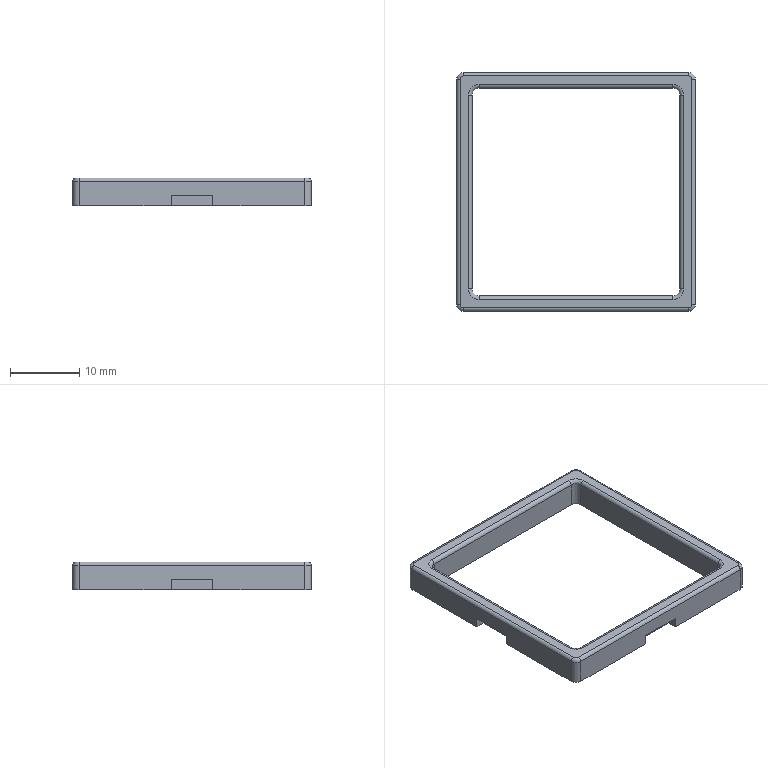Part | SolidWorks | features BaseBody 1 | 1 solid | 50 faces | box 34.5 x 34.5 x 4 mm | volume 1097 mm3 | plane 26 | cylinder 16 | torus 8 | commonest cylinder face diameters 1 x8 2 x8
STEP:
#1=CARTESIAN_POINT('',(3.,-17.25,1.5));
#2=VERTEX_POINT('',#1);
#3=CARTESIAN_POINT('',(-3.,-17.25,1.5));
#4=VERTEX_POINT('',#3);
#5=CARTESIAN_POINT('',(3.,-17.25,1.5));
#6=DIRECTION('',(-1.,0.,0.));
#7=VECTOR('',#6,1000.);
#8=LINE('',#5,#7);
#9=EDGE_CURVE('',#2,#4,#8,.T.);
#10=ORIENTED_EDGE('',*,*,#9,.T.);
#11=CARTESIAN_POINT('',(-3.,-15.85,1.5));
#12=VERTEX_POINT('',#11);
#13=CARTESIAN_POINT('',(-3.,-17.25,1.5));
#14=DIRECTION('',(0.,1.,0.));
#15=VECTOR('',#14,1000.);
#16=LINE('',#13,#15);
#17=EDGE_CURVE('',#4,#12,#16,.T.);
#18=ORIENTED_EDGE('',*,*,#17,.T.);
#19=CARTESIAN_POINT('',(3.,-15.85,1.5));
#20=VERTEX_POINT('',#19);
#21=CARTESIAN_POINT('',(3.,-15.85,1.5));
#22=DIRECTION('',(1.,0.,0.));
#23=VECTOR('',#22,1000.);
#24=LINE('',#21,#23);
#25=EDGE_CURVE('',#12,#20,#24,.T.);
#26=ORIENTED_EDGE('',*,*,#25,.T.);
#27=CARTESIAN_POINT('',(3.,-17.25,1.5));
#28=DIRECTION('',(0.,-1.,0.));
#29=VECTOR('',#28,1000.);
#30=LINE('',#27,#29);
#31=EDGE_CURVE('',#20,#2,#30,.T.);
#32=ORIENTED_EDGE('',*,*,#31,.T.);
#33=EDGE_LOOP('',(#10,#18,#26,#32));
#34=FACE_OUTER_BOUND('',#33,.T.);
#35=CARTESIAN_POINT('',(-3.,-17.25,1.5));
#36=DIRECTION('',(0.,0.,-1.));
#37=DIRECTION('',(0.,-1.,0.));
#38=AXIS2_PLACEMENT_3D('',#35,#36,#37);
#39=PLANE('',#38);
#40=ADVANCED_FACE('',(#34),#39,.T.);
#41=CARTESIAN_POINT('',(-3.,-17.25,0.));
#42=VERTEX_POINT('',#41);
#43=CARTESIAN_POINT('',(-3.,-15.85,0.));
#44=VERTEX_POINT('',#43);
#45=CARTESIAN_POINT('',(-3.,-17.25,0.));
#46=DIRECTION('',(0.,1.,0.));
#47=VECTOR('',#46,1000.);
#48=LINE('',#45,#47);
#49=EDGE_CURVE('',#42,#44,#48,.T.);
#50=ORIENTED_EDGE('',*,*,#49,.T.);
#51=CARTESIAN_POINT('',(-3.,-15.85,1.5));
#52=DIRECTION('',(0.,0.,-1.));
#53=VECTOR('',#52,1000.);
#54=LINE('',#51,#53);
#55=EDGE_CURVE('',#12,#44,#54,.T.);
#56=ORIENTED_EDGE('',*,*,#55,.F.);
#57=ORIENTED_EDGE('',*,*,#17,.F.);
#58=CARTESIAN_POINT('',(-3.,-17.25,1.5));
#59=DIRECTION('',(0.,0.,-1.));
#60=VECTOR('',#59,1000.);
#61=LINE('',#58,#60);
#62=EDGE_CURVE('',#4,#42,#61,.T.);
#63=ORIENTED_EDGE('',*,*,#62,.T.);
#64=EDGE_LOOP('',(#50,#56,#57,#63));
#65=FACE_OUTER_BOUND('',#64,.T.);
#66=CARTESIAN_POINT('',(-3.,-17.25,1.5));
#67=DIRECTION('',(-1.,0.,0.));
#68=DIRECTION('',(0.,1.,0.));
#69=AXIS2_PLACEMENT_3D('',#66,#67,#68);
#70=PLANE('',#69);
#71=ADVANCED_FACE('',(#65),#70,.F.);
#72=CARTESIAN_POINT('',(3.,-15.85,0.));
#73=VERTEX_POINT('',#72);
#74=CARTESIAN_POINT('',(3.,-15.85,0.));
#75=DIRECTION('',(1.,0.,0.));
#76=VECTOR('',#75,1000.);
#77=LINE('',#74,#76);
#78=EDGE_CURVE('',#44,#73,#77,.T.);
#79=ORIENTED_EDGE('',*,*,#78,.T.);
#80=CARTESIAN_POINT('',(3.,-15.85,1.5));
#81=DIRECTION('',(0.,0.,-1.));
#82=VECTOR('',#81,1000.);
#83=LINE('',#80,#82);
#84=EDGE_CURVE('',#20,#73,#83,.T.);
#85=ORIENTED_EDGE('',*,*,#84,.F.);
#86=ORIENTED_EDGE('',*,*,#25,.F.);
#87=ORIENTED_EDGE('',*,*,#55,.T.);
#88=EDGE_LOOP('',(#79,#85,#86,#87));
#89=FACE_OUTER_BOUND('',#88,.T.);
#90=CARTESIAN_POINT('',(3.,-15.85,1.5));
#91=DIRECTION('',(0.,1.,0.));
#92=DIRECTION('',(1.,0.,0.));
#93=AXIS2_PLACEMENT_3D('',#90,#91,#92);
#94=PLANE('',#93);
#95=ADVANCED_FACE('',(#89),#94,.F.);
#96=CARTESIAN_POINT('',(3.,-17.25,0.));
#97=VERTEX_POINT('',#96);
#98=CARTESIAN_POINT('',(3.,-17.25,0.));
#99=DIRECTION('',(0.,-1.,0.));
#100=VECTOR('',#99,1000.);
#101=LINE('',#98,#100);
#102=EDGE_CURVE('',#73,#97,#101,.T.);
#103=ORIENTED_EDGE('',*,*,#102,.T.);
#104=CARTESIAN_POINT('',(3.,-17.25,1.5));
#105=DIRECTION('',(0.,0.,-1.));
#106=VECTOR('',#105,1000.);
#107=LINE('',#104,#106);
#108=EDGE_CURVE('',#2,#97,#107,.T.);
#109=ORIENTED_EDGE('',*,*,#108,.F.);
#110=ORIENTED_EDGE('',*,*,#31,.F.);
#111=ORIENTED_EDGE('',*,*,#84,.T.);
#112=EDGE_LOOP('',(#103,#109,#110,#111));
#113=FACE_OUTER_BOUND('',#112,.T.);
#114=CARTESIAN_POINT('',(3.,-17.25,1.5));
#115=DIRECTION('',(1.,0.,0.));
#116=DIRECTION('',(0.,-1.,0.));
#117=AXIS2_PLACEMENT_3D('',#114,#115,#116);
#118=PLANE('',#117);
#119=ADVANCED_FACE('',(#113),#118,.F.);
#120=CARTESIAN_POINT('',(15.85,3.,1.5));
#121=VERTEX_POINT('',#120);
#122=CARTESIAN_POINT('',(17.25,3.,1.5));
#123=VERTEX_POINT('',#122);
#124=CARTESIAN_POINT('',(17.25,3.,1.5));
#125=DIRECTION('',(1.,0.,0.));
#126=VECTOR('',#125,1000.);
#127=LINE('',#124,#126);
#128=EDGE_CURVE('',#121,#123,#127,.T.);
#129=ORIENTED_EDGE('',*,*,#128,.T.);
#130=CARTESIAN_POINT('',(17.25,-3.,1.5));
#131=VERTEX_POINT('',#130);
#132=CARTESIAN_POINT('',(17.25,3.,1.5));
#133=DIRECTION('',(0.,-1.,0.));
#134=VECTOR('',#133,1000.);
#135=LINE('',#132,#134);
#136=EDGE_CURVE('',#123,#131,#135,.T.);
#137=ORIENTED_EDGE('',*,*,#136,.T.);
#138=CARTESIAN_POINT('',(15.85,-3.,1.5));
#139=VERTEX_POINT('',#138);
#140=CARTESIAN_POINT('',(17.25,-3.,1.5));
#141=DIRECTION('',(-1.,0.,0.));
#142=VECTOR('',#141,1000.);
#143=LINE('',#140,#142);
#144=EDGE_CURVE('',#131,#139,#143,.T.);
#145=ORIENTED_EDGE('',*,*,#144,.T.);
#146=CARTESIAN_POINT('',(15.85,3.,1.5));
#147=DIRECTION('',(0.,1.,0.));
#148=VECTOR('',#147,1000.);
#149=LINE('',#146,#148);
#150=EDGE_CURVE('',#139,#121,#149,.T.);
#151=ORIENTED_EDGE('',*,*,#150,.T.);
#152=EDGE_LOOP('',(#129,#137,#145,#151));
#153=FACE_OUTER_BOUND('',#152,.T.);
#154=CARTESIAN_POINT('',(15.85,3.,1.5));
#155=DIRECTION('',(0.,0.,1.));
#156=DIRECTION('',(1.,0.,0.));
#157=AXIS2_PLACEMENT_3D('',#154,#155,#156);
#158=PLANE('',#157);
#159=ADVANCED_FACE('',(#153),#158,.F.);
#160=CARTESIAN_POINT('',(17.25,-3.,0.));
#161=VERTEX_POINT('',#160);
#162=CARTESIAN_POINT('',(15.85,-3.,0.));
#163=VERTEX_POINT('',#162);
#164=CARTESIAN_POINT('',(17.25,-3.,0.));
#165=DIRECTION('',(-1.,0.,0.));
#166=VECTOR('',#165,1000.);
#167=LINE('',#164,#166);
#168=EDGE_CURVE('',#161,#163,#167,.T.);
#169=ORIENTED_EDGE('',*,*,#168,.T.);
#170=CARTESIAN_POINT('',(15.85,-3.,1.5));
#171=DIRECTION('',(0.,0.,-1.));
#172=VECTOR('',#171,1000.);
#173=LINE('',#170,#172);
#174=EDGE_CURVE('',#139,#163,#173,.T.);
#175=ORIENTED_EDGE('',*,*,#174,.F.);
#176=ORIENTED_EDGE('',*,*,#144,.F.);
#177=CARTESIAN_POINT('',(17.25,-3.,1.5));
#178=DIRECTION('',(0.,0.,-1.));
#179=VECTOR('',#178,1000.);
#180=LINE('',#177,#179);
#181=EDGE_CURVE('',#131,#161,#180,.T.);
#182=ORIENTED_EDGE('',*,*,#181,.T.);
#183=EDGE_LOOP('',(#169,#175,#176,#182));
#184=FACE_OUTER_BOUND('',#183,.T.);
#185=CARTESIAN_POINT('',(17.25,-3.,1.5));
#186=DIRECTION('',(0.,-1.,0.));
#187=DIRECTION('',(0.,0.,-1.));
#188=AXIS2_PLACEMENT_3D('',#185,#186,#187);
#189=PLANE('',#188);
#190=ADVANCED_FACE('',(#184),#189,.F.);
#191=CARTESIAN_POINT('',(15.85,3.,0.));
#192=VERTEX_POINT('',#191);
#193=CARTESIAN_POINT('',(15.85,3.,0.));
#194=DIRECTION('',(0.,1.,0.));
#195=VECTOR('',#194,1000.);
#196=LINE('',#193,#195);
#197=EDGE_CURVE('',#163,#192,#196,.T.);
#198=ORIENTED_EDGE('',*,*,#197,.T.);
#199=CARTESIAN_POINT('',(15.85,3.,1.5));
#200=DIRECTION('',(0.,0.,-1.));
#201=VECTOR('',#200,1000.);
#202=LINE('',#199,#201);
#203=EDGE_CURVE('',#121,#192,#202,.T.);
#204=ORIENTED_EDGE('',*,*,#203,.F.);
#205=ORIENTED_EDGE('',*,*,#150,.F.);
#206=ORIENTED_EDGE('',*,*,#174,.T.);
#207=EDGE_LOOP('',(#198,#204,#205,#206));
#208=FACE_OUTER_BOUND('',#207,.T.);
#209=CARTESIAN_POINT('',(15.85,3.,1.5));
#210=DIRECTION('',(-1.,0.,0.));
#211=DIRECTION('',(0.,0.,1.));
#212=AXIS2_PLACEMENT_3D('',#209,#210,#211);
#213=PLANE('',#212);
#214=ADVANCED_FACE('',(#208),#213,.F.);
#215=CARTESIAN_POINT('',(17.25,3.,0.));
#216=VERTEX_POINT('',#215);
#217=CARTESIAN_POINT('',(17.25,3.,0.));
#218=DIRECTION('',(1.,0.,0.));
#219=VECTOR('',#218,1000.);
#220=LINE('',#217,#219);
#221=EDGE_CURVE('',#192,#216,#220,.T.);
#222=ORIENTED_EDGE('',*,*,#221,.T.);
#223=CARTESIAN_POINT('',(17.25,3.,1.5));
#224=DIRECTION('',(0.,0.,-1.));
#225=VECTOR('',#224,1000.);
#226=LINE('',#223,#225);
#227=EDGE_CURVE('',#123,#216,#226,.T.);
#228=ORIENTED_EDGE('',*,*,#227,.F.);
#229=ORIENTED_EDGE('',*,*,#128,.F.);
#230=ORIENTED_EDGE('',*,*,#203,.T.);
#231=EDGE_LOOP('',(#222,#228,#229,#230));
#232=FACE_OUTER_BOUND('',#231,.T.);
#233=CARTESIAN_POINT('',(17.25,3.,1.5));
#234=DIRECTION('',(0.,1.,0.));
#235=DIRECTION('',(1.,0.,0.));
#236=AXIS2_PLACEMENT_3D('',#233,#234,#235);
#237=PLANE('',#236);
#238=ADVANCED_FACE('',(#232),#237,.F.);
#239=CARTESIAN_POINT('',(-17.25,-3.,1.5));
#240=VERTEX_POINT('',#239);
#241=CARTESIAN_POINT('',(-17.25,3.,1.5));
#242=VERTEX_POINT('',#241);
#243=CARTESIAN_POINT('',(-17.25,3.,1.5));
#244=DIRECTION('',(0.,1.,0.));
#245=VECTOR('',#244,1000.);
#246=LINE('',#243,#245);
#247=EDGE_CURVE('',#240,#242,#246,.T.);
#248=ORIENTED_EDGE('',*,*,#247,.T.);
#249=CARTESIAN_POINT('',(-15.85,3.,1.5));
#250=VERTEX_POINT('',#249);
#251=CARTESIAN_POINT('',(-17.25,3.,1.5));
#252=DIRECTION('',(1.,0.,0.));
#253=VECTOR('',#252,1000.);
#254=LINE('',#251,#253);
#255=EDGE_CURVE('',#242,#250,#254,.T.);
#256=ORIENTED_EDGE('',*,*,#255,.T.);
#257=CARTESIAN_POINT('',(-15.85,-3.,1.5));
#258=VERTEX_POINT('',#257);
#259=CARTESIAN_POINT('',(-15.85,3.,1.5));
#260=DIRECTION('',(0.,-1.,0.));
#261=VECTOR('',#260,1000.);
#262=LINE('',#259,#261);
#263=EDGE_CURVE('',#250,#258,#262,.T.);
#264=ORIENTED_EDGE('',*,*,#263,.T.);
#265=CARTESIAN_POINT('',(-17.25,-3.,1.5));
#266=DIRECTION('',(-1.,0.,0.));
#267=VECTOR('',#266,1000.);
#268=LINE('',#265,#267);
#269=EDGE_CURVE('',#258,#240,#268,.T.);
#270=ORIENTED_EDGE('',*,*,#269,.T.);
#271=EDGE_LOOP('',(#248,#256,#264,#270));
#272=FACE_OUTER_BOUND('',#271,.T.);
#273=CARTESIAN_POINT('',(-17.25,-3.,1.5));
#274=DIRECTION('',(0.,0.,1.));
#275=DIRECTION('',(1.,0.,0.));
#276=AXIS2_PLACEMENT_3D('',#273,#274,#275);
#277=PLANE('',#276);
#278=ADVANCED_FACE('',(#272),#277,.F.);
#279=CARTESIAN_POINT('',(-17.25,3.,0.));
#280=VERTEX_POINT('',#279);
#281=CARTESIAN_POINT('',(-15.85,3.,0.));
#282=VERTEX_POINT('',#281);
#283=CARTESIAN_POINT('',(-17.25,3.,0.));
#284=DIRECTION('',(1.,0.,0.));
#285=VECTOR('',#284,1000.);
#286=LINE('',#283,#285);
#287=EDGE_CURVE('',#280,#282,#286,.T.);
#288=ORIENTED_EDGE('',*,*,#287,.T.);
#289=CARTESIAN_POINT('',(-15.85,3.,1.5));
#290=DIRECTION('',(0.,0.,-1.));
#291=VECTOR('',#290,1000.);
#292=LINE('',#289,#291);
#293=EDGE_CURVE('',#250,#282,#292,.T.);
#294=ORIENTED_EDGE('',*,*,#293,.F.);
#295=ORIENTED_EDGE('',*,*,#255,.F.);
#296=CARTESIAN_POINT('',(-17.25,3.,1.5));
#297=DIRECTION('',(0.,0.,-1.));
#298=VECTOR('',#297,1000.);
#299=LINE('',#296,#298);
#300=EDGE_CURVE('',#242,#280,#299,.T.);
#301=ORIENTED_EDGE('',*,*,#300,.T.);
#302=EDGE_LOOP('',(#288,#294,#295,#301));
#303=FACE_OUTER_BOUND('',#302,.T.);
#304=CARTESIAN_POINT('',(-17.25,3.,1.5));
#305=DIRECTION('',(0.,1.,0.));
#306=DIRECTION('',(1.,0.,0.));
#307=AXIS2_PLACEMENT_3D('',#304,#305,#306);
#308=PLANE('',#307);
#309=ADVANCED_FACE('',(#303),#308,.F.);
#310=CARTESIAN_POINT('',(-15.85,-3.,0.));
#311=VERTEX_POINT('',#310);
#312=CARTESIAN_POINT('',(-15.85,3.,0.));
#313=DIRECTION('',(0.,-1.,0.));
#314=VECTOR('',#313,1000.);
#315=LINE('',#312,#314);
#316=EDGE_CURVE('',#282,#311,#315,.T.);
#317=ORIENTED_EDGE('',*,*,#316,.T.);
#318=CARTESIAN_POINT('',(-15.85,-3.,1.5));
#319=DIRECTION('',(0.,0.,-1.));
#320=VECTOR('',#319,1000.);
#321=LINE('',#318,#320);
#322=EDGE_CURVE('',#258,#311,#321,.T.);
#323=ORIENTED_EDGE('',*,*,#322,.F.);
#324=ORIENTED_EDGE('',*,*,#263,.F.);
#325=ORIENTED_EDGE('',*,*,#293,.T.);
#326=EDGE_LOOP('',(#317,#323,#324,#325));
#327=FACE_OUTER_BOUND('',#326,.T.);
#328=CARTESIAN_POINT('',(-15.85,3.,1.5));
#329=DIRECTION('',(1.,0.,0.));
#330=DIRECTION('',(0.,1.,0.));
#331=AXIS2_PLACEMENT_3D('',#328,#329,#330);
#332=PLANE('',#331);
#333=ADVANCED_FACE('',(#327),#332,.F.);
#334=CARTESIAN_POINT('',(-17.25,-3.,0.));
#335=VERTEX_POINT('',#334);
#336=CARTESIAN_POINT('',(-17.25,-3.,0.));
#337=DIRECTION('',(-1.,0.,0.));
#338=VECTOR('',#337,1000.);
#339=LINE('',#336,#338);
#340=EDGE_CURVE('',#311,#335,#339,.T.);
#341=ORIENTED_EDGE('',*,*,#340,.T.);
#342=CARTESIAN_POINT('',(-17.25,-3.,1.5));
#343=DIRECTION('',(0.,0.,-1.));
#344=VECTOR('',#343,1000.);
#345=LINE('',#342,#344);
#346=EDGE_CURVE('',#240,#335,#345,.T.);
#347=ORIENTED_EDGE('',*,*,#346,.F.);
#348=ORIENTED_EDGE('',*,*,#269,.F.);
#349=ORIENTED_EDGE('',*,*,#322,.T.);
#350=EDGE_LOOP('',(#341,#347,#348,#349));
#351=FACE_OUTER_BOUND('',#350,.T.);
#352=CARTESIAN_POINT('',(-17.25,-3.,1.5));
#353=DIRECTION('',(0.,-1.,0.));
#354=DIRECTION('',(-1.,0.,0.));
#355=AXIS2_PLACEMENT_3D('',#352,#353,#354);
#356=PLANE('',#355);
#357=ADVANCED_FACE('',(#351),#356,.F.);
#358=CARTESIAN_POINT('',(3.,17.25,1.5));
#359=VERTEX_POINT('',#358);
#360=CARTESIAN_POINT('',(3.,15.85,1.5));
#361=VERTEX_POINT('',#360);
#362=CARTESIAN_POINT('',(3.,17.25,1.5));
#363=DIRECTION('',(0.,-1.,0.));
#364=VECTOR('',#363,1000.);
#365=LINE('',#362,#364);
#366=EDGE_CURVE('',#359,#361,#365,.T.);
#367=ORIENTED_EDGE('',*,*,#366,.T.);
#368=CARTESIAN_POINT('',(-3.,15.85,1.5));
#369=VERTEX_POINT('',#368);
#370=CARTESIAN_POINT('',(3.,15.85,1.5));
#371=DIRECTION('',(-1.,0.,0.));
#372=VECTOR('',#371,1000.);
#373=LINE('',#370,#372);
#374=EDGE_CURVE('',#361,#369,#373,.T.);
#375=ORIENTED_EDGE('',*,*,#374,.T.);
#376=CARTESIAN_POINT('',(-3.,17.25,1.5));
#377=VERTEX_POINT('',#376);
#378=CARTESIAN_POINT('',(-3.,17.25,1.5));
#379=DIRECTION('',(0.,1.,0.));
#380=VECTOR('',#379,1000.);
#381=LINE('',#378,#380);
#382=EDGE_CURVE('',#369,#377,#381,.T.);
#383=ORIENTED_EDGE('',*,*,#382,.T.);
#384=CARTESIAN_POINT('',(3.,17.25,1.5));
#385=DIRECTION('',(1.,0.,0.));
#386=VECTOR('',#385,1000.);
#387=LINE('',#384,#386);
#388=EDGE_CURVE('',#377,#359,#387,.T.);
#389=ORIENTED_EDGE('',*,*,#388,.T.);
#390=EDGE_LOOP('',(#367,#375,#383,#389));
#391=FACE_OUTER_BOUND('',#390,.T.);
#392=CARTESIAN_POINT('',(3.,15.85,1.5));
#393=DIRECTION('',(0.,0.,-1.));
#394=DIRECTION('',(0.,-1.,0.));
#395=AXIS2_PLACEMENT_3D('',#392,#393,#394);
#396=PLANE('',#395);
#397=ADVANCED_FACE('',(#391),#396,.T.);
#398=CARTESIAN_POINT('',(3.,15.85,0.));
#399=VERTEX_POINT('',#398);
#400=CARTESIAN_POINT('',(-3.,15.85,0.));
#401=VERTEX_POINT('',#400);
#402=CARTESIAN_POINT('',(3.,15.85,0.));
#403=DIRECTION('',(-1.,0.,0.));
#404=VECTOR('',#403,1000.);
#405=LINE('',#402,#404);
#406=EDGE_CURVE('',#399,#401,#405,.T.);
#407=ORIENTED_EDGE('',*,*,#406,.T.);
#408=CARTESIAN_POINT('',(-3.,15.85,1.5));
#409=DIRECTION('',(0.,0.,-1.));
#410=VECTOR('',#409,1000.);
#411=LINE('',#408,#410);
#412=EDGE_CURVE('',#369,#401,#411,.T.);
#413=ORIENTED_EDGE('',*,*,#412,.F.);
#414=ORIENTED_EDGE('',*,*,#374,.F.);
#415=CARTESIAN_POINT('',(3.,15.85,1.5));
#416=DIRECTION('',(0.,0.,-1.));
#417=VECTOR('',#416,1000.);
#418=LINE('',#415,#417);
#419=EDGE_CURVE('',#361,#399,#418,.T.);
#420=ORIENTED_EDGE('',*,*,#419,.T.);
#421=EDGE_LOOP('',(#407,#413,#414,#420));
#422=FACE_OUTER_BOUND('',#421,.T.);
#423=CARTESIAN_POINT('',(3.,15.85,1.5));
#424=DIRECTION('',(0.,-1.,0.));
#425=DIRECTION('',(0.,0.,-1.));
#426=AXIS2_PLACEMENT_3D('',#423,#424,#425);
#427=PLANE('',#426);
#428=ADVANCED_FACE('',(#422),#427,.F.);
#429=CARTESIAN_POINT('',(-3.,17.25,0.));
#430=VERTEX_POINT('',#429);
#431=CARTESIAN_POINT('',(-3.,17.25,0.));
#432=DIRECTION('',(0.,1.,0.));
#433=VECTOR('',#432,1000.);
#434=LINE('',#431,#433);
#435=EDGE_CURVE('',#401,#430,#434,.T.);
#436=ORIENTED_EDGE('',*,*,#435,.T.);
#437=CARTESIAN_POINT('',(-3.,17.25,1.5));
#438=DIRECTION('',(0.,0.,-1.));
#439=VECTOR('',#438,1000.);
#440=LINE('',#437,#439);
#441=EDGE_CURVE('',#377,#430,#440,.T.);
#442=ORIENTED_EDGE('',*,*,#441,.F.);
#443=ORIENTED_EDGE('',*,*,#382,.F.);
#444=ORIENTED_EDGE('',*,*,#412,.T.);
#445=EDGE_LOOP('',(#436,#442,#443,#444));
#446=FACE_OUTER_BOUND('',#445,.T.);
#447=CARTESIAN_POINT('',(-3.,17.25,1.5));
#448=DIRECTION('',(-1.,0.,0.));
#449=DIRECTION('',(0.,0.,1.));
#450=AXIS2_PLACEMENT_3D('',#447,#448,#449);
#451=PLANE('',#450);
#452=ADVANCED_FACE('',(#446),#451,.F.);
#453=CARTESIAN_POINT('',(3.,17.25,0.));
#454=VERTEX_POINT('',#453);
#455=CARTESIAN_POINT('',(3.,17.25,0.));
#456=DIRECTION('',(0.,-1.,0.));
#457=VECTOR('',#456,1000.);
#458=LINE('',#455,#457);
#459=EDGE_CURVE('',#454,#399,#458,.T.);
#460=ORIENTED_EDGE('',*,*,#459,.T.);
#461=ORIENTED_EDGE('',*,*,#419,.F.);
#462=ORIENTED_EDGE('',*,*,#366,.F.);
#463=CARTESIAN_POINT('',(3.,17.25,1.5));
#464=DIRECTION('',(0.,0.,-1.));
#465=VECTOR('',#464,1000.);
#466=LINE('',#463,#465);
#467=EDGE_CURVE('',#359,#454,#466,.T.);
#468=ORIENTED_EDGE('',*,*,#467,.T.);
#469=EDGE_LOOP('',(#460,#461,#462,#468));
#470=FACE_OUTER_BOUND('',#469,.T.);
#471=CARTESIAN_POINT('',(3.,17.25,1.5));
#472=DIRECTION('',(1.,0.,0.));
#473=DIRECTION('',(0.,1.,0.));
#474=AXIS2_PLACEMENT_3D('',#471,#472,#473);
#475=PLANE('',#474);
#476=ADVANCED_FACE('',(#470),#475,.F.);
#477=CARTESIAN_POINT('',(-16.75,-16.25,4.));
#478=VERTEX_POINT('',#477);
#479=CARTESIAN_POINT('',(-17.25,-16.25,3.5));
#480=VERTEX_POINT('',#479);
#481=CARTESIAN_POINT('',(-16.75,-16.25,3.5));
#482=DIRECTION('',(0.,-1.,0.));
#483=DIRECTION('',(0.,0.,-1.));
#484=AXIS2_PLACEMENT_3D('',#481,#482,#483);
#485=CIRCLE('',#484,0.5);
#486=EDGE_CURVE('',#478,#480,#485,.T.);
#487=ORIENTED_EDGE('',*,*,#486,.T.);
#488=CARTESIAN_POINT('',(-16.25,-17.25,3.5));
#489=VERTEX_POINT('',#488);
#490=CARTESIAN_POINT('',(-16.25,-16.25,3.5));
#491=DIRECTION('',(0.,0.,-1.));
#492=DIRECTION('',(1.,0.,0.));
#493=AXIS2_PLACEMENT_3D('',#490,#491,#492);
#494=CIRCLE('',#493,1.);
#495=EDGE_CURVE('',#489,#480,#494,.T.);
#496=ORIENTED_EDGE('',*,*,#495,.F.);
#497=CARTESIAN_POINT('',(-16.25,-16.75,4.));
#498=VERTEX_POINT('',#497);
#499=CARTESIAN_POINT('',(-16.25,-16.75,3.5));
#500=DIRECTION('',(-1.,0.,0.));
#501=DIRECTION('',(0.,0.,1.));
#502=AXIS2_PLACEMENT_3D('',#499,#500,#501);
#503=CIRCLE('',#502,0.5);
#504=EDGE_CURVE('',#489,#498,#503,.T.);
#505=ORIENTED_EDGE('',*,*,#504,.T.);
#506=CARTESIAN_POINT('',(-16.25,-16.25,4.));
#507=DIRECTION('',(0.,0.,1.));
#508=DIRECTION('',(1.,0.,0.));
#509=AXIS2_PLACEMENT_3D('',#506,#507,#508);
#510=CIRCLE('',#509,0.5);
#511=EDGE_CURVE('',#478,#498,#510,.T.);
#512=ORIENTED_EDGE('',*,*,#511,.F.);
#513=EDGE_LOOP('',(#487,#496,#505,#512));
#514=FACE_OUTER_BOUND('',#513,.T.);
#515=CARTESIAN_POINT('',(-16.25,-16.25,3.5));
#516=DIRECTION('',(0.,0.,1.));
#517=DIRECTION('',(1.,0.,0.));
#518=AXIS2_PLACEMENT_3D('',#515,#516,#517);
#519=TOROIDAL_SURFACE('',#518,0.5,0.5);
#520=ADVANCED_FACE('',(#514),#519,.T.);
#521=CARTESIAN_POINT('',(16.25,-17.25,3.5));
#522=VERTEX_POINT('',#521);
#523=CARTESIAN_POINT('',(16.25,-16.75,4.));
#524=VERTEX_POINT('',#523);
#525=CARTESIAN_POINT('',(16.25,-16.75,3.5));
#526=DIRECTION('',(-1.,0.,0.));
#527=DIRECTION('',(0.,0.,1.));
#528=AXIS2_PLACEMENT_3D('',#525,#526,#527);
#529=CIRCLE('',#528,0.5);
#530=EDGE_CURVE('',#522,#524,#529,.T.);
#531=ORIENTED_EDGE('',*,*,#530,.T.);
#532=CARTESIAN_POINT('',(16.25,-16.75,4.));
#533=DIRECTION('',(1.,0.,0.));
#534=VECTOR('',#533,1000.);
#535=LINE('',#532,#534);
#536=EDGE_CURVE('',#498,#524,#535,.T.);
#537=ORIENTED_EDGE('',*,*,#536,.F.);
#538=ORIENTED_EDGE('',*,*,#504,.F.);
#539=CARTESIAN_POINT('',(-16.25,-17.25,3.5));
#540=DIRECTION('',(-1.,0.,0.));
#541=VECTOR('',#540,1000.);
#542=LINE('',#539,#541);
#543=EDGE_CURVE('',#522,#489,#542,.T.);
#544=ORIENTED_EDGE('',*,*,#543,.F.);
#545=EDGE_LOOP('',(#531,#537,#538,#544));
#546=FACE_OUTER_BOUND('',#545,.T.);
#547=CARTESIAN_POINT('',(-17.25,-16.75,3.5));
#548=DIRECTION('',(-1.,0.,0.));
#549=DIRECTION('',(0.,0.,1.));
#550=AXIS2_PLACEMENT_3D('',#547,#548,#549);
#551=CYLINDRICAL_SURFACE('',#550,0.5);
#552=ADVANCED_FACE('',(#546),#551,.T.);
#553=CARTESIAN_POINT('',(-16.75,16.25,4.));
#554=VERTEX_POINT('',#553);
#555=CARTESIAN_POINT('',(-17.25,16.25,3.5));
#556=VERTEX_POINT('',#555);
#557=CARTESIAN_POINT('',(-16.75,16.25,3.5));
#558=DIRECTION('',(0.,-1.,0.));
#559=DIRECTION('',(0.,0.,-1.));
#560=AXIS2_PLACEMENT_3D('',#557,#558,#559);
#561=CIRCLE('',#560,0.5);
#562=EDGE_CURVE('',#554,#556,#561,.T.);
#563=ORIENTED_EDGE('',*,*,#562,.T.);
#564=CARTESIAN_POINT('',(-17.25,16.25,3.5));
#565=DIRECTION('',(0.,1.,0.));
#566=VECTOR('',#565,1000.);
#567=LINE('',#564,#566);
#568=EDGE_CURVE('',#480,#556,#567,.T.);
#569=ORIENTED_EDGE('',*,*,#568,.F.);
#570=ORIENTED_EDGE('',*,*,#486,.F.);
#571=CARTESIAN_POINT('',(-16.75,-16.25,4.));
#572=DIRECTION('',(0.,-1.,0.));
#573=VECTOR('',#572,1000.);
#574=LINE('',#571,#573);
#575=EDGE_CURVE('',#554,#478,#574,.T.);
#576=ORIENTED_EDGE('',*,*,#575,.F.);
#577=EDGE_LOOP('',(#563,#569,#570,#576));
#578=FACE_OUTER_BOUND('',#577,.T.);
#579=CARTESIAN_POINT('',(-16.75,-17.25,3.5));
#580=DIRECTION('',(0.,1.,0.));
#581=DIRECTION('',(0.,0.,1.));
#582=AXIS2_PLACEMENT_3D('',#579,#580,#581);
#583=CYLINDRICAL_SURFACE('',#582,0.5);
#584=ADVANCED_FACE('',(#578),#583,.T.);
#585=CARTESIAN_POINT('',(17.25,-16.25,3.5));
#586=VERTEX_POINT('',#585);
#587=CARTESIAN_POINT('',(16.75,-16.25,4.));
#588=VERTEX_POINT('',#587);
#589=CARTESIAN_POINT('',(16.75,-16.25,3.5));
#590=DIRECTION('',(0.,-1.,0.));
#591=DIRECTION('',(0.,0.,-1.));
#592=AXIS2_PLACEMENT_3D('',#589,#590,#591);
#593=CIRCLE('',#592,0.5);
#594=EDGE_CURVE('',#586,#588,#593,.T.);
#595=ORIENTED_EDGE('',*,*,#594,.T.);
#596=CARTESIAN_POINT('',(16.25,-16.25,4.));
#597=DIRECTION('',(0.,0.,1.));
#598=DIRECTION('',(1.,0.,0.));
#599=AXIS2_PLACEMENT_3D('',#596,#597,#598);
#600=CIRCLE('',#599,0.5);
#601=EDGE_CURVE('',#524,#588,#600,.T.);
#602=ORIENTED_EDGE('',*,*,#601,.F.);
#603=ORIENTED_EDGE('',*,*,#530,.F.);
#604=CARTESIAN_POINT('',(16.25,-16.25,3.5));
#605=DIRECTION('',(0.,0.,-1.));
#606=DIRECTION('',(1.,0.,0.));
#607=AXIS2_PLACEMENT_3D('',#604,#605,#606);
#608=CIRCLE('',#607,1.);
#609=EDGE_CURVE('',#586,#522,#608,.T.);
#610=ORIENTED_EDGE('',*,*,#609,.F.);
#611=EDGE_LOOP('',(#595,#602,#603,#610));
#612=FACE_OUTER_BOUND('',#611,.T.);
#613=CARTESIAN_POINT('',(16.25,-16.25,3.5));
#614=DIRECTION('',(0.,0.,1.));
#615=DIRECTION('',(1.,0.,0.));
#616=AXIS2_PLACEMENT_3D('',#613,#614,#615);
#617=TOROIDAL_SURFACE('',#616,0.5,0.5);
#618=ADVANCED_FACE('',(#612),#617,.T.);
#619=CARTESIAN_POINT('',(-16.25,16.75,4.));
#620=VERTEX_POINT('',#619);
#621=CARTESIAN_POINT('',(-16.25,17.25,3.5));
#622=VERTEX_POINT('',#621);
#623=CARTESIAN_POINT('',(-16.25,16.75,3.5));
#624=DIRECTION('',(-1.,0.,0.));
#625=DIRECTION('',(0.,0.,1.));
#626=AXIS2_PLACEMENT_3D('',#623,#624,#625);
#627=CIRCLE('',#626,0.5);
#628=EDGE_CURVE('',#620,#622,#627,.T.);
#629=ORIENTED_EDGE('',*,*,#628,.T.);
#630=CARTESIAN_POINT('',(-16.25,16.25,3.5));
#631=DIRECTION('',(0.,0.,-1.));
#632=DIRECTION('',(1.,0.,0.));
#633=AXIS2_PLACEMENT_3D('',#630,#631,#632);
#634=CIRCLE('',#633,1.);
#635=EDGE_CURVE('',#556,#622,#634,.T.);
#636=ORIENTED_EDGE('',*,*,#635,.F.);
#637=ORIENTED_EDGE('',*,*,#562,.F.);
#638=CARTESIAN_POINT('',(-16.25,16.25,4.));
#639=DIRECTION('',(0.,0.,1.));
#640=DIRECTION('',(1.,0.,0.));
#641=AXIS2_PLACEMENT_3D('',#638,#639,#640);
#642=CIRCLE('',#641,0.5);
#643=EDGE_CURVE('',#620,#554,#642,.T.);
#644=ORIENTED_EDGE('',*,*,#643,.F.);
#645=EDGE_LOOP('',(#629,#636,#637,#644));
#646=FACE_OUTER_BOUND('',#645,.T.);
#647=CARTESIAN_POINT('',(-16.25,16.25,3.5));
#648=DIRECTION('',(0.,0.,1.));
#649=DIRECTION('',(1.,0.,0.));
#650=AXIS2_PLACEMENT_3D('',#647,#648,#649);
#651=TOROIDAL_SURFACE('',#650,0.5,0.5);
#652=ADVANCED_FACE('',(#646),#651,.T.);
#653=CARTESIAN_POINT('',(17.25,16.25,3.5));
#654=VERTEX_POINT('',#653);
#655=CARTESIAN_POINT('',(16.75,16.25,4.));
#656=VERTEX_POINT('',#655);
#657=CARTESIAN_POINT('',(16.75,16.25,3.5));
#658=DIRECTION('',(0.,-1.,0.));
#659=DIRECTION('',(0.,0.,-1.));
#660=AXIS2_PLACEMENT_3D('',#657,#658,#659);
#661=CIRCLE('',#660,0.5);
#662=EDGE_CURVE('',#654,#656,#661,.T.);
#663=ORIENTED_EDGE('',*,*,#662,.T.);
#664=CARTESIAN_POINT('',(16.75,16.25,4.));
#665=DIRECTION('',(0.,1.,0.));
#666=VECTOR('',#665,1000.);
#667=LINE('',#664,#666);
#668=EDGE_CURVE('',#588,#656,#667,.T.);
#669=ORIENTED_EDGE('',*,*,#668,.F.);
#670=ORIENTED_EDGE('',*,*,#594,.F.);
#671=CARTESIAN_POINT('',(17.25,-16.25,3.5));
#672=DIRECTION('',(0.,-1.,0.));
#673=VECTOR('',#672,1000.);
#674=LINE('',#671,#673);
#675=EDGE_CURVE('',#654,#586,#674,.T.);
#676=ORIENTED_EDGE('',*,*,#675,.F.);
#677=EDGE_LOOP('',(#663,#669,#670,#676));
#678=FACE_OUTER_BOUND('',#677,.T.);
#679=CARTESIAN_POINT('',(16.75,-17.25,3.5));
#680=DIRECTION('',(0.,-1.,0.));
#681=DIRECTION('',(1.,0.,0.));
#682=AXIS2_PLACEMENT_3D('',#679,#680,#681);
#683=CYLINDRICAL_SURFACE('',#682,0.5);
#684=ADVANCED_FACE('',(#678),#683,.T.);
#685=CARTESIAN_POINT('',(16.25,16.75,4.));
#686=VERTEX_POINT('',#685);
#687=CARTESIAN_POINT('',(16.25,17.25,3.5));
#688=VERTEX_POINT('',#687);
#689=CARTESIAN_POINT('',(16.25,16.75,3.5));
#690=DIRECTION('',(-1.,0.,0.));
#691=DIRECTION('',(0.,0.,1.));
#692=AXIS2_PLACEMENT_3D('',#689,#690,#691);
#693=CIRCLE('',#692,0.5);
#694=EDGE_CURVE('',#686,#688,#693,.T.);
#695=ORIENTED_EDGE('',*,*,#694,.T.);
#696=CARTESIAN_POINT('',(16.25,17.25,3.5));
#697=DIRECTION('',(1.,0.,0.));
#698=VECTOR('',#697,1000.);
#699=LINE('',#696,#698);
#700=EDGE_CURVE('',#622,#688,#699,.T.);
#701=ORIENTED_EDGE('',*,*,#700,.F.);
#702=ORIENTED_EDGE('',*,*,#628,.F.);
#703=CARTESIAN_POINT('',(-16.25,16.75,4.));
#704=DIRECTION('',(-1.,0.,0.));
#705=VECTOR('',#704,1000.);
#706=LINE('',#703,#705);
#707=EDGE_CURVE('',#686,#620,#706,.T.);
#708=ORIENTED_EDGE('',*,*,#707,.F.);
#709=EDGE_LOOP('',(#695,#701,#702,#708));
#710=FACE_OUTER_BOUND('',#709,.T.);
#711=CARTESIAN_POINT('',(-17.25,16.75,3.5));
#712=DIRECTION('',(1.,0.,0.));
#713=DIRECTION('',(0.,0.,-1.));
#714=AXIS2_PLACEMENT_3D('',#711,#712,#713);
#715=CYLINDRICAL_SURFACE('',#714,0.5);
#716=ADVANCED_FACE('',(#710),#715,.T.);
#717=ORIENTED_EDGE('',*,*,#662,.F.);
#718=CARTESIAN_POINT('',(16.25,16.25,3.5));
#719=DIRECTION('',(0.,0.,-1.));
#720=DIRECTION('',(1.,0.,0.));
#721=AXIS2_PLACEMENT_3D('',#718,#719,#720);
#722=CIRCLE('',#721,1.);
#723=EDGE_CURVE('',#688,#654,#722,.T.);
#724=ORIENTED_EDGE('',*,*,#723,.F.);
#725=ORIENTED_EDGE('',*,*,#694,.F.);
#726=CARTESIAN_POINT('',(16.25,16.25,4.));
#727=DIRECTION('',(0.,0.,1.));
#728=DIRECTION('',(1.,0.,0.));
#729=AXIS2_PLACEMENT_3D('',#726,#727,#728);
#730=CIRCLE('',#729,0.5);
#731=EDGE_CURVE('',#656,#686,#730,.T.);
#732=ORIENTED_EDGE('',*,*,#731,.F.);
#733=EDGE_LOOP('',(#717,#724,#725,#732));
#734=FACE_OUTER_BOUND('',#733,.T.);
#735=CARTESIAN_POINT('',(16.25,16.25,3.5));
#736=DIRECTION('',(0.,0.,1.));
#737=DIRECTION('',(1.,0.,0.));
#738=AXIS2_PLACEMENT_3D('',#735,#736,#737);
#739=TOROIDAL_SURFACE('',#738,0.5,0.5);
#740=ADVANCED_FACE('',(#734),#739,.T.);
#741=CARTESIAN_POINT('',(15.5,-14.,4.));
#742=VERTEX_POINT('',#741);
#743=CARTESIAN_POINT('',(15.,-14.,3.5));
#744=VERTEX_POINT('',#743);
#745=CARTESIAN_POINT('',(15.5,-14.,3.5));
#746=DIRECTION('',(0.,-1.,0.));
#747=DIRECTION('',(0.,0.,-1.));
#748=AXIS2_PLACEMENT_3D('',#745,#746,#747);
#749=CIRCLE('',#748,0.5);
#750=EDGE_CURVE('',#742,#744,#749,.T.);
#751=ORIENTED_EDGE('',*,*,#750,.T.);
#752=CARTESIAN_POINT('',(14.,-15.,3.5));
#753=VERTEX_POINT('',#752);
#754=CARTESIAN_POINT('',(14.,-14.,3.5));
#755=DIRECTION('',(0.,0.,1.));
#756=DIRECTION('',(1.,0.,0.));
#757=AXIS2_PLACEMENT_3D('',#754,#755,#756);
#758=CIRCLE('',#757,1.);
#759=EDGE_CURVE('',#753,#744,#758,.T.);
#760=ORIENTED_EDGE('',*,*,#759,.F.);
#761=CARTESIAN_POINT('',(14.,-15.5,4.));
#762=VERTEX_POINT('',#761);
#763=CARTESIAN_POINT('',(14.,-15.5,3.5));
#764=DIRECTION('',(1.,0.,0.));
#765=DIRECTION('',(0.,0.,-1.));
#766=AXIS2_PLACEMENT_3D('',#763,#764,#765);
#767=CIRCLE('',#766,0.5);
#768=EDGE_CURVE('',#753,#762,#767,.T.);
#769=ORIENTED_EDGE('',*,*,#768,.T.);
#770=CARTESIAN_POINT('',(14.,-14.,4.));
#771=DIRECTION('',(0.,0.,-1.));
#772=DIRECTION('',(1.,0.,0.));
#773=AXIS2_PLACEMENT_3D('',#770,#771,#772);
#774=CIRCLE('',#773,1.5);
#775=EDGE_CURVE('',#742,#762,#774,.T.);
#776=ORIENTED_EDGE('',*,*,#775,.F.);
#777=EDGE_LOOP('',(#751,#760,#769,#776));
#778=FACE_OUTER_BOUND('',#777,.T.);
#779=CARTESIAN_POINT('',(14.,-14.,3.5));
#780=DIRECTION('',(0.,0.,1.));
#781=DIRECTION('',(1.,0.,0.));
#782=AXIS2_PLACEMENT_3D('',#779,#780,#781);
#783=TOROIDAL_SURFACE('',#782,1.5,0.5);
#784=ADVANCED_FACE('',(#778),#783,.T.);
#785=CARTESIAN_POINT('',(-14.,-15.,3.5));
#786=VERTEX_POINT('',#785);
#787=CARTESIAN_POINT('',(-14.,-15.5,4.));
#788=VERTEX_POINT('',#787);
#789=CARTESIAN_POINT('',(-14.,-15.5,3.5));
#790=DIRECTION('',(1.,0.,0.));
#791=DIRECTION('',(0.,0.,-1.));
#792=AXIS2_PLACEMENT_3D('',#789,#790,#791);
#793=CIRCLE('',#792,0.5);
#794=EDGE_CURVE('',#786,#788,#793,.T.);
#795=ORIENTED_EDGE('',*,*,#794,.T.);
#796=CARTESIAN_POINT('',(-17.25,-15.5,4.));
#797=DIRECTION('',(-1.,0.,0.));
#798=VECTOR('',#797,1000.);
#799=LINE('',#796,#798);
#800=EDGE_CURVE('',#762,#788,#799,.T.);
#801=ORIENTED_EDGE('',*,*,#800,.F.);
#802=ORIENTED_EDGE('',*,*,#768,.F.);
#803=CARTESIAN_POINT('',(-15.,-15.,3.5));
#804=DIRECTION('',(1.,0.,0.));
#805=VECTOR('',#804,1000.);
#806=LINE('',#803,#805);
#807=EDGE_CURVE('',#786,#753,#806,.T.);
#808=ORIENTED_EDGE('',*,*,#807,.F.);
#809=EDGE_LOOP('',(#795,#801,#802,#808));
#810=FACE_OUTER_BOUND('',#809,.T.);
#811=CARTESIAN_POINT('',(-15.,-15.5,3.5));
#812=DIRECTION('',(1.,0.,0.));
#813=DIRECTION('',(0.,0.,-1.));
#814=AXIS2_PLACEMENT_3D('',#811,#812,#813);
#815=CYLINDRICAL_SURFACE('',#814,0.5);
#816=ADVANCED_FACE('',(#810),#815,.T.);
#817=CARTESIAN_POINT('',(15.5,14.,4.));
#818=VERTEX_POINT('',#817);
#819=CARTESIAN_POINT('',(15.,14.,3.5));
#820=VERTEX_POINT('',#819);
#821=CARTESIAN_POINT('',(15.5,14.,3.5));
#822=DIRECTION('',(0.,-1.,0.));
#823=DIRECTION('',(0.,0.,-1.));
#824=AXIS2_PLACEMENT_3D('',#821,#822,#823);
#825=CIRCLE('',#824,0.5);
#826=EDGE_CURVE('',#818,#820,#825,.T.);
#827=ORIENTED_EDGE('',*,*,#826,.T.);
#828=CARTESIAN_POINT('',(15.,-15.,3.5));
#829=DIRECTION('',(0.,1.,0.));
#830=VECTOR('',#829,1000.);
#831=LINE('',#828,#830);
#832=EDGE_CURVE('',#744,#820,#831,.T.);
#833=ORIENTED_EDGE('',*,*,#832,.F.);
#834=ORIENTED_EDGE('',*,*,#750,.F.);
#835=CARTESIAN_POINT('',(15.5,-17.25,4.));
#836=DIRECTION('',(0.,-1.,0.));
#837=VECTOR('',#836,1000.);
#838=LINE('',#835,#837);
#839=EDGE_CURVE('',#818,#742,#838,.T.);
#840=ORIENTED_EDGE('',*,*,#839,.F.);
#841=EDGE_LOOP('',(#827,#833,#834,#840));
#842=FACE_OUTER_BOUND('',#841,.T.);
#843=CARTESIAN_POINT('',(15.5,-15.,3.5));
#844=DIRECTION('',(0.,1.,0.));
#845=DIRECTION('',(-1.,0.,0.));
#846=AXIS2_PLACEMENT_3D('',#843,#844,#845);
#847=CYLINDRICAL_SURFACE('',#846,0.5);
#848=ADVANCED_FACE('',(#842),#847,.T.);
#849=CARTESIAN_POINT('',(-15.,-14.,3.5));
#850=VERTEX_POINT('',#849);
#851=CARTESIAN_POINT('',(-15.5,-14.,4.));
#852=VERTEX_POINT('',#851);
#853=CARTESIAN_POINT('',(-15.5,-14.,3.5));
#854=DIRECTION('',(0.,-1.,0.));
#855=DIRECTION('',(0.,0.,-1.));
#856=AXIS2_PLACEMENT_3D('',#853,#854,#855);
#857=CIRCLE('',#856,0.5);
#858=EDGE_CURVE('',#850,#852,#857,.T.);
#859=ORIENTED_EDGE('',*,*,#858,.T.);
#860=CARTESIAN_POINT('',(-14.,-14.,4.));
#861=DIRECTION('',(0.,0.,-1.));
#862=DIRECTION('',(1.,0.,0.));
#863=AXIS2_PLACEMENT_3D('',#860,#861,#862);
#864=CIRCLE('',#863,1.5);
#865=EDGE_CURVE('',#788,#852,#864,.T.);
#866=ORIENTED_EDGE('',*,*,#865,.F.);
#867=ORIENTED_EDGE('',*,*,#794,.F.);
#868=CARTESIAN_POINT('',(-14.,-14.,3.5));
#869=DIRECTION('',(0.,0.,1.));
#870=DIRECTION('',(1.,0.,0.));
#871=AXIS2_PLACEMENT_3D('',#868,#869,#870);
#872=CIRCLE('',#871,1.);
#873=EDGE_CURVE('',#850,#786,#872,.T.);
#874=ORIENTED_EDGE('',*,*,#873,.F.);
#875=EDGE_LOOP('',(#859,#866,#867,#874));
#876=FACE_OUTER_BOUND('',#875,.T.);
#877=CARTESIAN_POINT('',(-14.,-14.,3.5));
#878=DIRECTION('',(0.,0.,1.));
#879=DIRECTION('',(1.,0.,0.));
#880=AXIS2_PLACEMENT_3D('',#877,#878,#879);
#881=TOROIDAL_SURFACE('',#880,1.5,0.5);
#882=ADVANCED_FACE('',(#876),#881,.T.);
#883=CARTESIAN_POINT('',(14.,15.5,4.));
#884=VERTEX_POINT('',#883);
#885=CARTESIAN_POINT('',(14.,15.,3.5));
#886=VERTEX_POINT('',#885);
#887=CARTESIAN_POINT('',(14.,15.5,3.5));
#888=DIRECTION('',(1.,0.,0.));
#889=DIRECTION('',(0.,0.,-1.));
#890=AXIS2_PLACEMENT_3D('',#887,#888,#889);
#891=CIRCLE('',#890,0.5);
#892=EDGE_CURVE('',#884,#886,#891,.T.);
#893=ORIENTED_EDGE('',*,*,#892,.T.);
#894=CARTESIAN_POINT('',(14.,14.,3.5));
#895=DIRECTION('',(0.,0.,1.));
#896=DIRECTION('',(1.,0.,0.));
#897=AXIS2_PLACEMENT_3D('',#894,#895,#896);
#898=CIRCLE('',#897,1.);
#899=EDGE_CURVE('',#820,#886,#898,.T.);
#900=ORIENTED_EDGE('',*,*,#899,.F.);
#901=ORIENTED_EDGE('',*,*,#826,.F.);
#902=CARTESIAN_POINT('',(14.,14.,4.));
#903=DIRECTION('',(0.,0.,-1.));
#904=DIRECTION('',(1.,0.,0.));
#905=AXIS2_PLACEMENT_3D('',#902,#903,#904);
#906=CIRCLE('',#905,1.5);
#907=EDGE_CURVE('',#884,#818,#906,.T.);
#908=ORIENTED_EDGE('',*,*,#907,.F.);
#909=EDGE_LOOP('',(#893,#900,#901,#908));
#910=FACE_OUTER_BOUND('',#909,.T.);
#911=CARTESIAN_POINT('',(14.,14.,3.5));
#912=DIRECTION('',(0.,0.,1.));
#913=DIRECTION('',(1.,0.,0.));
#914=AXIS2_PLACEMENT_3D('',#911,#912,#913);
#915=TOROIDAL_SURFACE('',#914,1.5,0.5);
#916=ADVANCED_FACE('',(#910),#915,.T.);
#917=CARTESIAN_POINT('',(-15.,14.,3.5));
#918=VERTEX_POINT('',#917);
#919=CARTESIAN_POINT('',(-15.5,14.,4.));
#920=VERTEX_POINT('',#919);
#921=CARTESIAN_POINT('',(-15.5,14.,3.5));
#922=DIRECTION('',(0.,-1.,0.));
#923=DIRECTION('',(0.,0.,-1.));
#924=AXIS2_PLACEMENT_3D('',#921,#922,#923);
#925=CIRCLE('',#924,0.5);
#926=EDGE_CURVE('',#918,#920,#925,.T.);
#927=ORIENTED_EDGE('',*,*,#926,.T.);
#928=CARTESIAN_POINT('',(-15.5,-17.25,4.));
#929=DIRECTION('',(0.,1.,0.));
#930=VECTOR('',#929,1000.);
#931=LINE('',#928,#930);
#932=EDGE_CURVE('',#852,#920,#931,.T.);
#933=ORIENTED_EDGE('',*,*,#932,.F.);
#934=ORIENTED_EDGE('',*,*,#858,.F.);
#935=CARTESIAN_POINT('',(-15.,-15.,3.5));
#936=DIRECTION('',(0.,-1.,0.));
#937=VECTOR('',#936,1000.);
#938=LINE('',#935,#937);
#939=EDGE_CURVE('',#918,#850,#938,.T.);
#940=ORIENTED_EDGE('',*,*,#939,.F.);
#941=EDGE_LOOP('',(#927,#933,#934,#940));
#942=FACE_OUTER_BOUND('',#941,.T.);
#943=CARTESIAN_POINT('',(-15.5,-15.,3.5));
#944=DIRECTION('',(0.,-1.,0.));
#945=DIRECTION('',(0.,0.,-1.));
#946=AXIS2_PLACEMENT_3D('',#943,#944,#945);
#947=CYLINDRICAL_SURFACE('',#946,0.5);
#948=ADVANCED_FACE('',(#942),#947,.T.);
#949=CARTESIAN_POINT('',(-14.,15.5,4.));
#950=VERTEX_POINT('',#949);
#951=CARTESIAN_POINT('',(-14.,15.,3.5));
#952=VERTEX_POINT('',#951);
#953=CARTESIAN_POINT('',(-14.,15.5,3.5));
#954=DIRECTION('',(1.,0.,0.));
#955=DIRECTION('',(0.,0.,-1.));
#956=AXIS2_PLACEMENT_3D('',#953,#954,#955);
#957=CIRCLE('',#956,0.5);
#958=EDGE_CURVE('',#950,#952,#957,.T.);
#959=ORIENTED_EDGE('',*,*,#958,.T.);
#960=CARTESIAN_POINT('',(-15.,15.,3.5));
#961=DIRECTION('',(-1.,0.,0.));
#962=VECTOR('',#961,1000.);
#963=LINE('',#960,#962);
#964=EDGE_CURVE('',#886,#952,#963,.T.);
#965=ORIENTED_EDGE('',*,*,#964,.F.);
#966=ORIENTED_EDGE('',*,*,#892,.F.);
#967=CARTESIAN_POINT('',(-17.25,15.5,4.));
#968=DIRECTION('',(1.,0.,0.));
#969=VECTOR('',#968,1000.);
#970=LINE('',#967,#969);
#971=EDGE_CURVE('',#950,#884,#970,.T.);
#972=ORIENTED_EDGE('',*,*,#971,.F.);
#973=EDGE_LOOP('',(#959,#965,#966,#972));
#974=FACE_OUTER_BOUND('',#973,.T.);
#975=CARTESIAN_POINT('',(-15.,15.5,3.5));
#976=DIRECTION('',(-1.,0.,0.));
#977=DIRECTION('',(0.,0.,1.));
#978=AXIS2_PLACEMENT_3D('',#975,#976,#977);
#979=CYLINDRICAL_SURFACE('',#978,0.5);
#980=ADVANCED_FACE('',(#974),#979,.T.);
#981=ORIENTED_EDGE('',*,*,#926,.F.);
#982=CARTESIAN_POINT('',(-14.,14.,3.5));
#983=DIRECTION('',(0.,0.,1.));
#984=DIRECTION('',(1.,0.,0.));
#985=AXIS2_PLACEMENT_3D('',#982,#983,#984);
#986=CIRCLE('',#985,1.);
#987=EDGE_CURVE('',#952,#918,#986,.T.);
#988=ORIENTED_EDGE('',*,*,#987,.F.);
#989=ORIENTED_EDGE('',*,*,#958,.F.);
#990=CARTESIAN_POINT('',(-14.,14.,4.));
#991=DIRECTION('',(0.,0.,-1.));
#992=DIRECTION('',(1.,0.,0.));
#993=AXIS2_PLACEMENT_3D('',#990,#991,#992);
#994=CIRCLE('',#993,1.5);
#995=EDGE_CURVE('',#920,#950,#994,.T.);
#996=ORIENTED_EDGE('',*,*,#995,.F.);
#997=EDGE_LOOP('',(#981,#988,#989,#996));
#998=FACE_OUTER_BOUND('',#997,.T.);
#999=CARTESIAN_POINT('',(-14.,14.,3.5));
#1000=DIRECTION('',(0.,0.,1.));
#1001=DIRECTION('',(1.,0.,0.));
#1002=AXIS2_PLACEMENT_3D('',#999,#1000,#1001);
#1003=TOROIDAL_SURFACE('',#1002,1.5,0.5);
#1004=ADVANCED_FACE('',(#998),#1003,.T.);
#1005=CARTESIAN_POINT('',(14.,-15.,0.));
#1006=VERTEX_POINT('',#1005);
#1007=CARTESIAN_POINT('',(14.,-15.,0.));
#1008=DIRECTION('',(0.,0.,-1.));
#1009=VECTOR('',#1008,1000.);
#1010=LINE('',#1007,#1009);
#1011=EDGE_CURVE('',#753,#1006,#1010,.T.);
#1012=ORIENTED_EDGE('',*,*,#1011,.F.);
#1013=ORIENTED_EDGE('',*,*,#759,.T.);
#1014=CARTESIAN_POINT('',(15.,-14.,0.));
#1015=VERTEX_POINT('',#1014);
#1016=CARTESIAN_POINT('',(15.,-14.,4.));
#1017=DIRECTION('',(0.,0.,1.));
#1018=VECTOR('',#1017,1000.);
#1019=LINE('',#1016,#1018);
#1020=EDGE_CURVE('',#1015,#744,#1019,.T.);
#1021=ORIENTED_EDGE('',*,*,#1020,.F.);
#1022=CARTESIAN_POINT('',(14.,-14.,0.));
#1023=DIRECTION('',(0.,0.,1.));
#1024=DIRECTION('',(1.,0.,0.));
#1025=AXIS2_PLACEMENT_3D('',#1022,#1023,#1024);
#1026=CIRCLE('',#1025,1.);
#1027=EDGE_CURVE('',#1006,#1015,#1026,.T.);
#1028=ORIENTED_EDGE('',*,*,#1027,.F.);
#1029=EDGE_LOOP('',(#1012,#1013,#1021,#1028));
#1030=FACE_OUTER_BOUND('',#1029,.T.);
#1031=CARTESIAN_POINT('',(14.,-14.,4.));
#1032=DIRECTION('',(0.,0.,1.));
#1033=DIRECTION('',(1.,0.,0.));
#1034=AXIS2_PLACEMENT_3D('',#1031,#1032,#1033);
#1035=CYLINDRICAL_SURFACE('',#1034,1.);
#1036=ADVANCED_FACE('',(#1030),#1035,.F.);
#1037=CARTESIAN_POINT('',(15.,14.,0.));
#1038=VERTEX_POINT('',#1037);
#1039=CARTESIAN_POINT('',(15.,14.,0.));
#1040=DIRECTION('',(0.,0.,-1.));
#1041=VECTOR('',#1040,1000.);
#1042=LINE('',#1039,#1041);
#1043=EDGE_CURVE('',#820,#1038,#1042,.T.);
#1044=ORIENTED_EDGE('',*,*,#1043,.F.);
#1045=ORIENTED_EDGE('',*,*,#899,.T.);
#1046=CARTESIAN_POINT('',(14.,15.,0.));
#1047=VERTEX_POINT('',#1046);
#1048=CARTESIAN_POINT('',(14.,15.,4.));
#1049=DIRECTION('',(0.,0.,1.));
#1050=VECTOR('',#1049,1000.);
#1051=LINE('',#1048,#1050);
#1052=EDGE_CURVE('',#1047,#886,#1051,.T.);
#1053=ORIENTED_EDGE('',*,*,#1052,.F.);
#1054=CARTESIAN_POINT('',(14.,14.,0.));
#1055=DIRECTION('',(0.,0.,1.));
#1056=DIRECTION('',(1.,0.,0.));
#1057=AXIS2_PLACEMENT_3D('',#1054,#1055,#1056);
#1058=CIRCLE('',#1057,1.);
#1059=EDGE_CURVE('',#1038,#1047,#1058,.T.);
#1060=ORIENTED_EDGE('',*,*,#1059,.F.);
#1061=EDGE_LOOP('',(#1044,#1045,#1053,#1060));
#1062=FACE_OUTER_BOUND('',#1061,.T.);
#1063=CARTESIAN_POINT('',(14.,14.,4.));
#1064=DIRECTION('',(0.,0.,1.));
#1065=DIRECTION('',(1.,0.,0.));
#1066=AXIS2_PLACEMENT_3D('',#1063,#1064,#1065);
#1067=CYLINDRICAL_SURFACE('',#1066,1.);
#1068=ADVANCED_FACE('',(#1062),#1067,.F.);
#1069=CARTESIAN_POINT('',(-14.,15.,0.));
#1070=VERTEX_POINT('',#1069);
#1071=CARTESIAN_POINT('',(-14.,15.,0.));
#1072=DIRECTION('',(0.,0.,-1.));
#1073=VECTOR('',#1072,1000.);
#1074=LINE('',#1071,#1073);
#1075=EDGE_CURVE('',#952,#1070,#1074,.T.);
#1076=ORIENTED_EDGE('',*,*,#1075,.F.);
#1077=ORIENTED_EDGE('',*,*,#987,.T.);
#1078=CARTESIAN_POINT('',(-15.,14.,0.));
#1079=VERTEX_POINT('',#1078);
#1080=CARTESIAN_POINT('',(-15.,14.,4.));
#1081=DIRECTION('',(0.,0.,1.));
#1082=VECTOR('',#1081,1000.);
#1083=LINE('',#1080,#1082);
#1084=EDGE_CURVE('',#1079,#918,#1083,.T.);
#1085=ORIENTED_EDGE('',*,*,#1084,.F.);
#1086=CARTESIAN_POINT('',(-14.,14.,0.));
#1087=DIRECTION('',(0.,0.,1.));
#1088=DIRECTION('',(1.,0.,0.));
#1089=AXIS2_PLACEMENT_3D('',#1086,#1087,#1088);
#1090=CIRCLE('',#1089,1.);
#1091=EDGE_CURVE('',#1070,#1079,#1090,.T.);
#1092=ORIENTED_EDGE('',*,*,#1091,.F.);
#1093=EDGE_LOOP('',(#1076,#1077,#1085,#1092));
#1094=FACE_OUTER_BOUND('',#1093,.T.);
#1095=CARTESIAN_POINT('',(-14.,14.,4.));
#1096=DIRECTION('',(0.,0.,1.));
#1097=DIRECTION('',(1.,0.,0.));
#1098=AXIS2_PLACEMENT_3D('',#1095,#1096,#1097);
#1099=CYLINDRICAL_SURFACE('',#1098,1.);
#1100=ADVANCED_FACE('',(#1094),#1099,.F.);
#1101=CARTESIAN_POINT('',(-15.,-14.,0.));
#1102=VERTEX_POINT('',#1101);
#1103=CARTESIAN_POINT('',(-15.,-14.,0.));
#1104=DIRECTION('',(0.,0.,-1.));
#1105=VECTOR('',#1104,1000.);
#1106=LINE('',#1103,#1105);
#1107=EDGE_CURVE('',#850,#1102,#1106,.T.);
#1108=ORIENTED_EDGE('',*,*,#1107,.F.);
#1109=ORIENTED_EDGE('',*,*,#873,.T.);
#1110=CARTESIAN_POINT('',(-14.,-15.,0.));
#1111=VERTEX_POINT('',#1110);
#1112=CARTESIAN_POINT('',(-14.,-15.,4.));
#1113=DIRECTION('',(0.,0.,1.));
#1114=VECTOR('',#1113,1000.);
#1115=LINE('',#1112,#1114);
#1116=EDGE_CURVE('',#1111,#786,#1115,.T.);
#1117=ORIENTED_EDGE('',*,*,#1116,.F.);
#1118=CARTESIAN_POINT('',(-14.,-14.,0.));
#1119=DIRECTION('',(0.,0.,1.));
#1120=DIRECTION('',(1.,0.,0.));
#1121=AXIS2_PLACEMENT_3D('',#1118,#1119,#1120);
#1122=CIRCLE('',#1121,1.);
#1123=EDGE_CURVE('',#1102,#1111,#1122,.T.);
#1124=ORIENTED_EDGE('',*,*,#1123,.F.);
#1125=EDGE_LOOP('',(#1108,#1109,#1117,#1124));
#1126=FACE_OUTER_BOUND('',#1125,.T.);
#1127=CARTESIAN_POINT('',(-14.,-14.,4.));
#1128=DIRECTION('',(0.,0.,1.));
#1129=DIRECTION('',(1.,0.,0.));
#1130=AXIS2_PLACEMENT_3D('',#1127,#1128,#1129);
#1131=CYLINDRICAL_SURFACE('',#1130,1.);
#1132=ADVANCED_FACE('',(#1126),#1131,.F.);
#1133=CARTESIAN_POINT('',(16.25,17.25,0.));
#1134=VERTEX_POINT('',#1133);
#1135=CARTESIAN_POINT('',(16.25,17.25,4.));
#1136=DIRECTION('',(0.,0.,-1.));
#1137=VECTOR('',#1136,1000.);
#1138=LINE('',#1135,#1137);
#1139=EDGE_CURVE('',#688,#1134,#1138,.T.);
#1140=ORIENTED_EDGE('',*,*,#1139,.F.);
#1141=ORIENTED_EDGE('',*,*,#723,.T.);
#1142=CARTESIAN_POINT('',(17.25,16.25,0.));
#1143=VERTEX_POINT('',#1142);
#1144=CARTESIAN_POINT('',(17.25,16.25,4.));
#1145=DIRECTION('',(0.,0.,1.));
#1146=VECTOR('',#1145,1000.);
#1147=LINE('',#1144,#1146);
#1148=EDGE_CURVE('',#1143,#654,#1147,.T.);
#1149=ORIENTED_EDGE('',*,*,#1148,.F.);
#1150=CARTESIAN_POINT('',(16.25,16.25,0.));
#1151=DIRECTION('',(0.,0.,-1.));
#1152=DIRECTION('',(1.,0.,0.));
#1153=AXIS2_PLACEMENT_3D('',#1150,#1151,#1152);
#1154=CIRCLE('',#1153,1.);
#1155=EDGE_CURVE('',#1134,#1143,#1154,.T.);
#1156=ORIENTED_EDGE('',*,*,#1155,.F.);
#1157=EDGE_LOOP('',(#1140,#1141,#1149,#1156));
#1158=FACE_OUTER_BOUND('',#1157,.T.);
#1159=CARTESIAN_POINT('',(16.25,16.25,4.));
#1160=DIRECTION('',(0.,0.,-1.));
#1161=DIRECTION('',(-1.,0.,0.));
#1162=AXIS2_PLACEMENT_3D('',#1159,#1160,#1161);
#1163=CYLINDRICAL_SURFACE('',#1162,1.);
#1164=ADVANCED_FACE('',(#1158),#1163,.T.);
#1165=CARTESIAN_POINT('',(-17.25,16.25,0.));
#1166=VERTEX_POINT('',#1165);
#1167=CARTESIAN_POINT('',(-17.25,16.25,4.));
#1168=DIRECTION('',(0.,0.,-1.));
#1169=VECTOR('',#1168,1000.);
#1170=LINE('',#1167,#1169);
#1171=EDGE_CURVE('',#556,#1166,#1170,.T.);
#1172=ORIENTED_EDGE('',*,*,#1171,.F.);
#1173=ORIENTED_EDGE('',*,*,#635,.T.);
#1174=CARTESIAN_POINT('',(-16.25,17.25,0.));
#1175=VERTEX_POINT('',#1174);
#1176=CARTESIAN_POINT('',(-16.25,17.25,4.));
#1177=DIRECTION('',(0.,0.,1.));
#1178=VECTOR('',#1177,1000.);
#1179=LINE('',#1176,#1178);
#1180=EDGE_CURVE('',#1175,#622,#1179,.T.);
#1181=ORIENTED_EDGE('',*,*,#1180,.F.);
#1182=CARTESIAN_POINT('',(-16.25,16.25,0.));
#1183=DIRECTION('',(0.,0.,-1.));
#1184=DIRECTION('',(1.,0.,0.));
#1185=AXIS2_PLACEMENT_3D('',#1182,#1183,#1184);
#1186=CIRCLE('',#1185,1.);
#1187=EDGE_CURVE('',#1166,#1175,#1186,.T.);
#1188=ORIENTED_EDGE('',*,*,#1187,.F.);
#1189=EDGE_LOOP('',(#1172,#1173,#1181,#1188));
#1190=FACE_OUTER_BOUND('',#1189,.T.);
#1191=CARTESIAN_POINT('',(-16.25,16.25,4.));
#1192=DIRECTION('',(0.,0.,-1.));
#1193=DIRECTION('',(-1.,0.,0.));
#1194=AXIS2_PLACEMENT_3D('',#1191,#1192,#1193);
#1195=CYLINDRICAL_SURFACE('',#1194,1.);
#1196=ADVANCED_FACE('',(#1190),#1195,.T.);
#1197=CARTESIAN_POINT('',(-16.25,-17.25,0.));
#1198=VERTEX_POINT('',#1197);
#1199=CARTESIAN_POINT('',(-16.25,-17.25,4.));
#1200=DIRECTION('',(0.,0.,-1.));
#1201=VECTOR('',#1200,1000.);
#1202=LINE('',#1199,#1201);
#1203=EDGE_CURVE('',#489,#1198,#1202,.T.);
#1204=ORIENTED_EDGE('',*,*,#1203,.F.);
#1205=ORIENTED_EDGE('',*,*,#495,.T.);
#1206=CARTESIAN_POINT('',(-17.25,-16.25,0.));
#1207=VERTEX_POINT('',#1206);
#1208=CARTESIAN_POINT('',(-17.25,-16.25,4.));
#1209=DIRECTION('',(0.,0.,1.));
#1210=VECTOR('',#1209,1000.);
#1211=LINE('',#1208,#1210);
#1212=EDGE_CURVE('',#1207,#480,#1211,.T.);
#1213=ORIENTED_EDGE('',*,*,#1212,.F.);
#1214=CARTESIAN_POINT('',(-16.25,-16.25,0.));
#1215=DIRECTION('',(0.,0.,-1.));
#1216=DIRECTION('',(1.,0.,0.));
#1217=AXIS2_PLACEMENT_3D('',#1214,#1215,#1216);
#1218=CIRCLE('',#1217,1.);
#1219=EDGE_CURVE('',#1198,#1207,#1218,.T.);
#1220=ORIENTED_EDGE('',*,*,#1219,.F.);
#1221=EDGE_LOOP('',(#1204,#1205,#1213,#1220));
#1222=FACE_OUTER_BOUND('',#1221,.T.);
#1223=CARTESIAN_POINT('',(-16.25,-16.25,4.));
#1224=DIRECTION('',(0.,0.,-1.));
#1225=DIRECTION('',(-1.,0.,0.));
#1226=AXIS2_PLACEMENT_3D('',#1223,#1224,#1225);
#1227=CYLINDRICAL_SURFACE('',#1226,1.);
#1228=ADVANCED_FACE('',(#1222),#1227,.T.);
#1229=CARTESIAN_POINT('',(17.25,-16.25,0.));
#1230=VERTEX_POINT('',#1229);
#1231=CARTESIAN_POINT('',(17.25,-16.25,4.));
#1232=DIRECTION('',(0.,0.,-1.));
#1233=VECTOR('',#1232,1000.);
#1234=LINE('',#1231,#1233);
#1235=EDGE_CURVE('',#586,#1230,#1234,.T.);
#1236=ORIENTED_EDGE('',*,*,#1235,.F.);
#1237=ORIENTED_EDGE('',*,*,#609,.T.);
#1238=CARTESIAN_POINT('',(16.25,-17.25,0.));
#1239=VERTEX_POINT('',#1238);
#1240=CARTESIAN_POINT('',(16.25,-17.25,4.));
#1241=DIRECTION('',(0.,0.,1.));
#1242=VECTOR('',#1241,1000.);
#1243=LINE('',#1240,#1242);
#1244=EDGE_CURVE('',#1239,#522,#1243,.T.);
#1245=ORIENTED_EDGE('',*,*,#1244,.F.);
#1246=CARTESIAN_POINT('',(16.25,-16.25,0.));
#1247=DIRECTION('',(0.,0.,-1.));
#1248=DIRECTION('',(1.,0.,0.));
#1249=AXIS2_PLACEMENT_3D('',#1246,#1247,#1248);
#1250=CIRCLE('',#1249,1.);
#1251=EDGE_CURVE('',#1230,#1239,#1250,.T.);
#1252=ORIENTED_EDGE('',*,*,#1251,.F.);
#1253=EDGE_LOOP('',(#1236,#1237,#1245,#1252));
#1254=FACE_OUTER_BOUND('',#1253,.T.);
#1255=CARTESIAN_POINT('',(16.25,-16.25,4.));
#1256=DIRECTION('',(0.,0.,-1.));
#1257=DIRECTION('',(-1.,0.,0.));
#1258=AXIS2_PLACEMENT_3D('',#1255,#1256,#1257);
#1259=CYLINDRICAL_SURFACE('',#1258,1.);
#1260=ADVANCED_FACE('',(#1254),#1259,.T.);
#1261=ORIENTED_EDGE('',*,*,#1052,.T.);
#1262=ORIENTED_EDGE('',*,*,#964,.T.);
#1263=ORIENTED_EDGE('',*,*,#1075,.T.);
#1264=CARTESIAN_POINT('',(-15.,15.,0.));
#1265=DIRECTION('',(-1.,0.,0.));
#1266=VECTOR('',#1265,1000.);
#1267=LINE('',#1264,#1266);
#1268=EDGE_CURVE('',#1047,#1070,#1267,.T.);
#1269=ORIENTED_EDGE('',*,*,#1268,.F.);
#1270=EDGE_LOOP('',(#1261,#1262,#1263,#1269));
#1271=FACE_OUTER_BOUND('',#1270,.T.);
#1272=CARTESIAN_POINT('',(-15.,15.,4.));
#1273=DIRECTION('',(0.,-1.,0.));
#1274=DIRECTION('',(0.,0.,-1.));
#1275=AXIS2_PLACEMENT_3D('',#1272,#1273,#1274);
#1276=PLANE('',#1275);
#1277=ADVANCED_FACE('',(#1271),#1276,.T.);
#1278=ORIENTED_EDGE('',*,*,#1020,.T.);
#1279=ORIENTED_EDGE('',*,*,#832,.T.);
#1280=ORIENTED_EDGE('',*,*,#1043,.T.);
#1281=CARTESIAN_POINT('',(15.,-15.,0.));
#1282=DIRECTION('',(0.,1.,0.));
#1283=VECTOR('',#1282,1000.);
#1284=LINE('',#1281,#1283);
#1285=EDGE_CURVE('',#1015,#1038,#1284,.T.);
#1286=ORIENTED_EDGE('',*,*,#1285,.F.);
#1287=EDGE_LOOP('',(#1278,#1279,#1280,#1286));
#1288=FACE_OUTER_BOUND('',#1287,.T.);
#1289=CARTESIAN_POINT('',(15.,-15.,4.));
#1290=DIRECTION('',(-1.,0.,0.));
#1291=DIRECTION('',(0.,0.,1.));
#1292=AXIS2_PLACEMENT_3D('',#1289,#1290,#1291);
#1293=PLANE('',#1292);
#1294=ADVANCED_FACE('',(#1288),#1293,.T.);
#1295=ORIENTED_EDGE('',*,*,#1116,.T.);
#1296=ORIENTED_EDGE('',*,*,#807,.T.);
#1297=ORIENTED_EDGE('',*,*,#1011,.T.);
#1298=CARTESIAN_POINT('',(-15.,-15.,0.));
#1299=DIRECTION('',(1.,0.,0.));
#1300=VECTOR('',#1299,1000.);
#1301=LINE('',#1298,#1300);
#1302=EDGE_CURVE('',#1111,#1006,#1301,.T.);
#1303=ORIENTED_EDGE('',*,*,#1302,.F.);
#1304=EDGE_LOOP('',(#1295,#1296,#1297,#1303));
#1305=FACE_OUTER_BOUND('',#1304,.T.);
#1306=CARTESIAN_POINT('',(-15.,-15.,4.));
#1307=DIRECTION('',(0.,1.,0.));
#1308=DIRECTION('',(1.,0.,0.));
#1309=AXIS2_PLACEMENT_3D('',#1306,#1307,#1308);
#1310=PLANE('',#1309);
#1311=ADVANCED_FACE('',(#1305),#1310,.T.);
#1312=ORIENTED_EDGE('',*,*,#1084,.T.);
#1313=ORIENTED_EDGE('',*,*,#939,.T.);
#1314=ORIENTED_EDGE('',*,*,#1107,.T.);
#1315=CARTESIAN_POINT('',(-15.,-15.,0.));
#1316=DIRECTION('',(0.,-1.,0.));
#1317=VECTOR('',#1316,1000.);
#1318=LINE('',#1315,#1317);
#1319=EDGE_CURVE('',#1079,#1102,#1318,.T.);
#1320=ORIENTED_EDGE('',*,*,#1319,.F.);
#1321=EDGE_LOOP('',(#1312,#1313,#1314,#1320));
#1322=FACE_OUTER_BOUND('',#1321,.T.);
#1323=CARTESIAN_POINT('',(-15.,-15.,4.));
#1324=DIRECTION('',(1.,0.,0.));
#1325=DIRECTION('',(0.,1.,0.));
#1326=AXIS2_PLACEMENT_3D('',#1323,#1324,#1325);
#1327=PLANE('',#1326);
#1328=ADVANCED_FACE('',(#1322),#1327,.T.);
#1329=CARTESIAN_POINT('',(-15.,17.25,0.));
#1330=DIRECTION('',(-1.,0.,0.));
#1331=VECTOR('',#1330,1000.);
#1332=LINE('',#1329,#1331);
#1333=EDGE_CURVE('',#1134,#454,#1332,.T.);
#1334=ORIENTED_EDGE('',*,*,#1333,.T.);
#1335=ORIENTED_EDGE('',*,*,#467,.F.);
#1336=ORIENTED_EDGE('',*,*,#388,.F.);
#1337=ORIENTED_EDGE('',*,*,#441,.T.);
#1338=CARTESIAN_POINT('',(-15.,17.25,0.));
#1339=DIRECTION('',(-1.,0.,0.));
#1340=VECTOR('',#1339,1000.);
#1341=LINE('',#1338,#1340);
#1342=EDGE_CURVE('',#430,#1175,#1341,.T.);
#1343=ORIENTED_EDGE('',*,*,#1342,.T.);
#1344=ORIENTED_EDGE('',*,*,#1180,.T.);
#1345=ORIENTED_EDGE('',*,*,#700,.T.);
#1346=ORIENTED_EDGE('',*,*,#1139,.T.);
#1347=EDGE_LOOP('',(#1334,#1335,#1336,#1337,#1343,#1344,#1345,#1346));
#1348=FACE_OUTER_BOUND('',#1347,.T.);
#1349=CARTESIAN_POINT('',(-15.,17.25,4.));
#1350=DIRECTION('',(0.,-1.,0.));
#1351=DIRECTION('',(0.,0.,-1.));
#1352=AXIS2_PLACEMENT_3D('',#1349,#1350,#1351);
#1353=PLANE('',#1352);
#1354=ADVANCED_FACE('',(#1348),#1353,.F.);
#1355=ORIENTED_EDGE('',*,*,#136,.F.);
#1356=ORIENTED_EDGE('',*,*,#227,.T.);
#1357=CARTESIAN_POINT('',(17.25,15.,0.));
#1358=DIRECTION('',(0.,1.,0.));
#1359=VECTOR('',#1358,1000.);
#1360=LINE('',#1357,#1359);
#1361=EDGE_CURVE('',#216,#1143,#1360,.T.);
#1362=ORIENTED_EDGE('',*,*,#1361,.T.);
#1363=ORIENTED_EDGE('',*,*,#1148,.T.);
#1364=ORIENTED_EDGE('',*,*,#675,.T.);
#1365=ORIENTED_EDGE('',*,*,#1235,.T.);
#1366=CARTESIAN_POINT('',(17.25,15.,0.));
#1367=DIRECTION('',(0.,1.,0.));
#1368=VECTOR('',#1367,1000.);
#1369=LINE('',#1366,#1368);
#1370=EDGE_CURVE('',#1230,#161,#1369,.T.);
#1371=ORIENTED_EDGE('',*,*,#1370,.T.);
#1372=ORIENTED_EDGE('',*,*,#181,.F.);
#1373=EDGE_LOOP('',(#1355,#1356,#1362,#1363,#1364,#1365,#1371,#1372));
#1374=FACE_OUTER_BOUND('',#1373,.T.);
#1375=CARTESIAN_POINT('',(17.25,15.,4.));
#1376=DIRECTION('',(-1.,0.,0.));
#1377=DIRECTION('',(0.,0.,1.));
#1378=AXIS2_PLACEMENT_3D('',#1375,#1376,#1377);
#1379=PLANE('',#1378);
#1380=ADVANCED_FACE('',(#1374),#1379,.F.);
#1381=ORIENTED_EDGE('',*,*,#9,.F.);
#1382=ORIENTED_EDGE('',*,*,#108,.T.);
#1383=CARTESIAN_POINT('',(-15.,-17.25,0.));
#1384=DIRECTION('',(1.,0.,0.));
#1385=VECTOR('',#1384,1000.);
#1386=LINE('',#1383,#1385);
#1387=EDGE_CURVE('',#97,#1239,#1386,.T.);
#1388=ORIENTED_EDGE('',*,*,#1387,.T.);
#1389=ORIENTED_EDGE('',*,*,#1244,.T.);
#1390=ORIENTED_EDGE('',*,*,#543,.T.);
#1391=ORIENTED_EDGE('',*,*,#1203,.T.);
#1392=CARTESIAN_POINT('',(-15.,-17.25,0.));
#1393=DIRECTION('',(1.,0.,0.));
#1394=VECTOR('',#1393,1000.);
#1395=LINE('',#1392,#1394);
#1396=EDGE_CURVE('',#1198,#42,#1395,.T.);
#1397=ORIENTED_EDGE('',*,*,#1396,.T.);
#1398=ORIENTED_EDGE('',*,*,#62,.F.);
#1399=EDGE_LOOP('',(#1381,#1382,#1388,#1389,#1390,#1391,#1397,#1398));
#1400=FACE_OUTER_BOUND('',#1399,.T.);
#1401=CARTESIAN_POINT('',(-15.,-17.25,4.));
#1402=DIRECTION('',(0.,1.,0.));
#1403=DIRECTION('',(1.,0.,0.));
#1404=AXIS2_PLACEMENT_3D('',#1401,#1402,#1403);
#1405=PLANE('',#1404);
#1406=ADVANCED_FACE('',(#1400),#1405,.F.);
#1407=ORIENTED_EDGE('',*,*,#247,.F.);
#1408=ORIENTED_EDGE('',*,*,#346,.T.);
#1409=CARTESIAN_POINT('',(-17.25,15.,0.));
#1410=DIRECTION('',(0.,-1.,0.));
#1411=VECTOR('',#1410,1000.);
#1412=LINE('',#1409,#1411);
#1413=EDGE_CURVE('',#335,#1207,#1412,.T.);
#1414=ORIENTED_EDGE('',*,*,#1413,.T.);
#1415=ORIENTED_EDGE('',*,*,#1212,.T.);
#1416=ORIENTED_EDGE('',*,*,#568,.T.);
#1417=ORIENTED_EDGE('',*,*,#1171,.T.);
#1418=CARTESIAN_POINT('',(-17.25,15.,0.));
#1419=DIRECTION('',(0.,-1.,0.));
#1420=VECTOR('',#1419,1000.);
#1421=LINE('',#1418,#1420);
#1422=EDGE_CURVE('',#1166,#280,#1421,.T.);
#1423=ORIENTED_EDGE('',*,*,#1422,.T.);
#1424=ORIENTED_EDGE('',*,*,#300,.F.);
#1425=EDGE_LOOP('',(#1407,#1408,#1414,#1415,#1416,#1417,#1423,#1424));
#1426=FACE_OUTER_BOUND('',#1425,.T.);
#1427=CARTESIAN_POINT('',(-17.25,15.,4.));
#1428=DIRECTION('',(1.,0.,0.));
#1429=DIRECTION('',(0.,1.,0.));
#1430=AXIS2_PLACEMENT_3D('',#1427,#1428,#1429);
#1431=PLANE('',#1430);
#1432=ADVANCED_FACE('',(#1426),#1431,.F.);
#1433=ORIENTED_EDGE('',*,*,#1268,.T.);
#1434=ORIENTED_EDGE('',*,*,#1091,.T.);
#1435=ORIENTED_EDGE('',*,*,#1319,.T.);
#1436=ORIENTED_EDGE('',*,*,#1123,.T.);
#1437=ORIENTED_EDGE('',*,*,#1302,.T.);
#1438=ORIENTED_EDGE('',*,*,#1027,.T.);
#1439=ORIENTED_EDGE('',*,*,#1285,.T.);
#1440=ORIENTED_EDGE('',*,*,#1059,.T.);
#1441=EDGE_LOOP('',(#1433,#1434,#1435,#1436,#1437,#1438,#1439,#1440));
#1442=FACE_BOUND('',#1441,.T.);
#1443=ORIENTED_EDGE('',*,*,#1387,.F.);
#1444=ORIENTED_EDGE('',*,*,#102,.F.);
#1445=ORIENTED_EDGE('',*,*,#78,.F.);
#1446=ORIENTED_EDGE('',*,*,#49,.F.);
#1447=ORIENTED_EDGE('',*,*,#1396,.F.);
#1448=ORIENTED_EDGE('',*,*,#1219,.T.);
#1449=ORIENTED_EDGE('',*,*,#1413,.F.);
#1450=ORIENTED_EDGE('',*,*,#340,.F.);
#1451=ORIENTED_EDGE('',*,*,#316,.F.);
#1452=ORIENTED_EDGE('',*,*,#287,.F.);
#1453=ORIENTED_EDGE('',*,*,#1422,.F.);
#1454=ORIENTED_EDGE('',*,*,#1187,.T.);
#1455=ORIENTED_EDGE('',*,*,#1342,.F.);
#1456=ORIENTED_EDGE('',*,*,#435,.F.);
#1457=ORIENTED_EDGE('',*,*,#406,.F.);
#1458=ORIENTED_EDGE('',*,*,#459,.F.);
#1459=ORIENTED_EDGE('',*,*,#1333,.F.);
#1460=ORIENTED_EDGE('',*,*,#1155,.T.);
#1461=ORIENTED_EDGE('',*,*,#1361,.F.);
#1462=ORIENTED_EDGE('',*,*,#221,.F.);
#1463=ORIENTED_EDGE('',*,*,#197,.F.);
#1464=ORIENTED_EDGE('',*,*,#168,.F.);
#1465=ORIENTED_EDGE('',*,*,#1370,.F.);
#1466=ORIENTED_EDGE('',*,*,#1251,.T.);
#1467=EDGE_LOOP('',(#1443,#1444,#1445,#1446,#1447,#1448,#1449,#1450,#1451,#1452,#1453,#1454,#1455,#1456,#1457,#1458,#1459,#1460,#1461,#1462,#1463,#1464,#1465,#1466));
#1468=FACE_OUTER_BOUND('',#1467,.T.);
#1469=CARTESIAN_POINT('',(-17.25,-17.25,0.));
#1470=DIRECTION('',(0.,0.,1.));
#1471=DIRECTION('',(1.,0.,0.));
#1472=AXIS2_PLACEMENT_3D('',#1469,#1470,#1471);
#1473=PLANE('',#1472);
#1474=ADVANCED_FACE('',(#1442,#1468),#1473,.F.);
#1475=ORIENTED_EDGE('',*,*,#839,.T.);
#1476=ORIENTED_EDGE('',*,*,#775,.T.);
#1477=ORIENTED_EDGE('',*,*,#800,.T.);
#1478=ORIENTED_EDGE('',*,*,#865,.T.);
#1479=ORIENTED_EDGE('',*,*,#932,.T.);
#1480=ORIENTED_EDGE('',*,*,#995,.T.);
#1481=ORIENTED_EDGE('',*,*,#971,.T.);
#1482=ORIENTED_EDGE('',*,*,#907,.T.);
#1483=EDGE_LOOP('',(#1475,#1476,#1477,#1478,#1479,#1480,#1481,#1482));
#1484=FACE_BOUND('',#1483,.T.);
#1485=ORIENTED_EDGE('',*,*,#575,.T.);
#1486=ORIENTED_EDGE('',*,*,#511,.T.);
#1487=ORIENTED_EDGE('',*,*,#536,.T.);
#1488=ORIENTED_EDGE('',*,*,#601,.T.);
#1489=ORIENTED_EDGE('',*,*,#668,.T.);
#1490=ORIENTED_EDGE('',*,*,#731,.T.);
#1491=ORIENTED_EDGE('',*,*,#707,.T.);
#1492=ORIENTED_EDGE('',*,*,#643,.T.);
#1493=EDGE_LOOP('',(#1485,#1486,#1487,#1488,#1489,#1490,#1491,#1492));
#1494=FACE_OUTER_BOUND('',#1493,.T.);
#1495=CARTESIAN_POINT('',(-17.25,-17.25,4.));
#1496=DIRECTION('',(0.,0.,1.));
#1497=DIRECTION('',(1.,0.,0.));
#1498=AXIS2_PLACEMENT_3D('',#1495,#1496,#1497);
#1499=PLANE('',#1498);
#1500=ADVANCED_FACE('',(#1484,#1494),#1499,.T.);
#1501=CLOSED_SHELL('',(#40,#71,#95,#119,#159,#190,#214,#238,#278,#309,#333,#357,#397,#428,#452,#476,#520,#552,#584,#618,#652,#684,#716,#740,#784,#816,#848,#882,#916,#948,#980,#1004,#1036,#1068,#1100,#1132,#1164,#1196,#1228,#1260,#1277,#1294,#1311,#1328,#1354,#1380,#1406,#1432,#1474,#1500));
#1502=MANIFOLD_SOLID_BREP('',#1501);
#1503=CARTESIAN_POINT('',(0.,0.,0.));
#1504=DIRECTION('',(0.,0.,1.));
#1505=DIRECTION('',(1.,0.,0.));
#1506=AXIS2_PLACEMENT_3D('',#1503,#1504,#1505);
#1507=(LENGTH_UNIT()NAMED_UNIT(*)SI_UNIT(.MILLI.,.METRE.));
#1508=UNCERTAINTY_MEASURE_WITH_UNIT(LENGTH_MEASURE(0.00001),#1507,'','');
#1509=(NAMED_UNIT(*)PLANE_ANGLE_UNIT()SI_UNIT($,.RADIAN.));
#1510=(NAMED_UNIT(*)SI_UNIT($,.STERADIAN.)SOLID_ANGLE_UNIT());
#1511=(GEOMETRIC_REPRESENTATION_CONTEXT(3)GLOBAL_UNCERTAINTY_ASSIGNED_CONTEXT((#1508))GLOBAL_UNIT_ASSIGNED_CONTEXT((#1507,#1509,#1510))REPRESENTATION_CONTEXT('',''));
#1512=ADVANCED_BREP_SHAPE_REPRESENTATION('',(#1502,#1506),#1511);